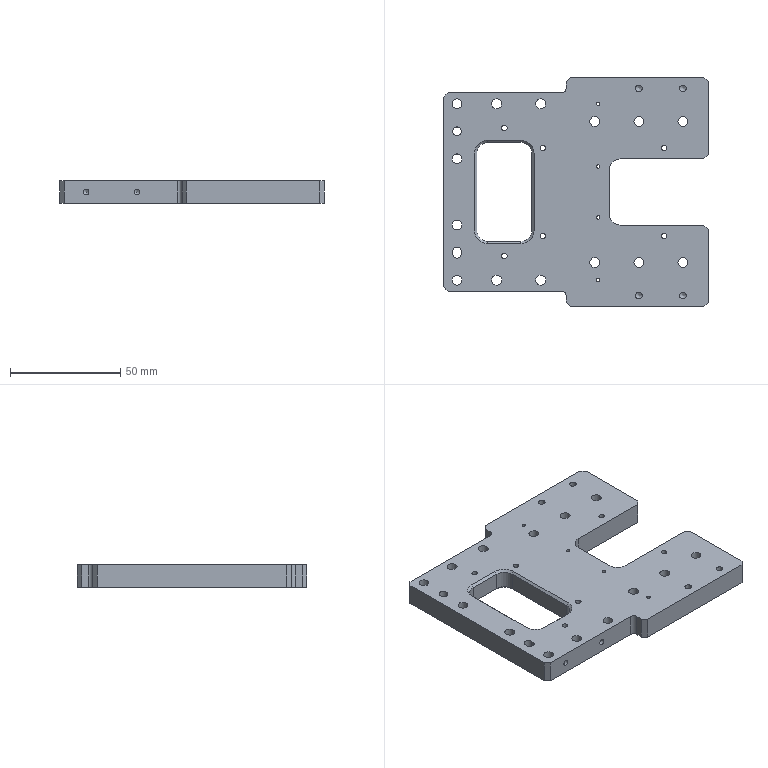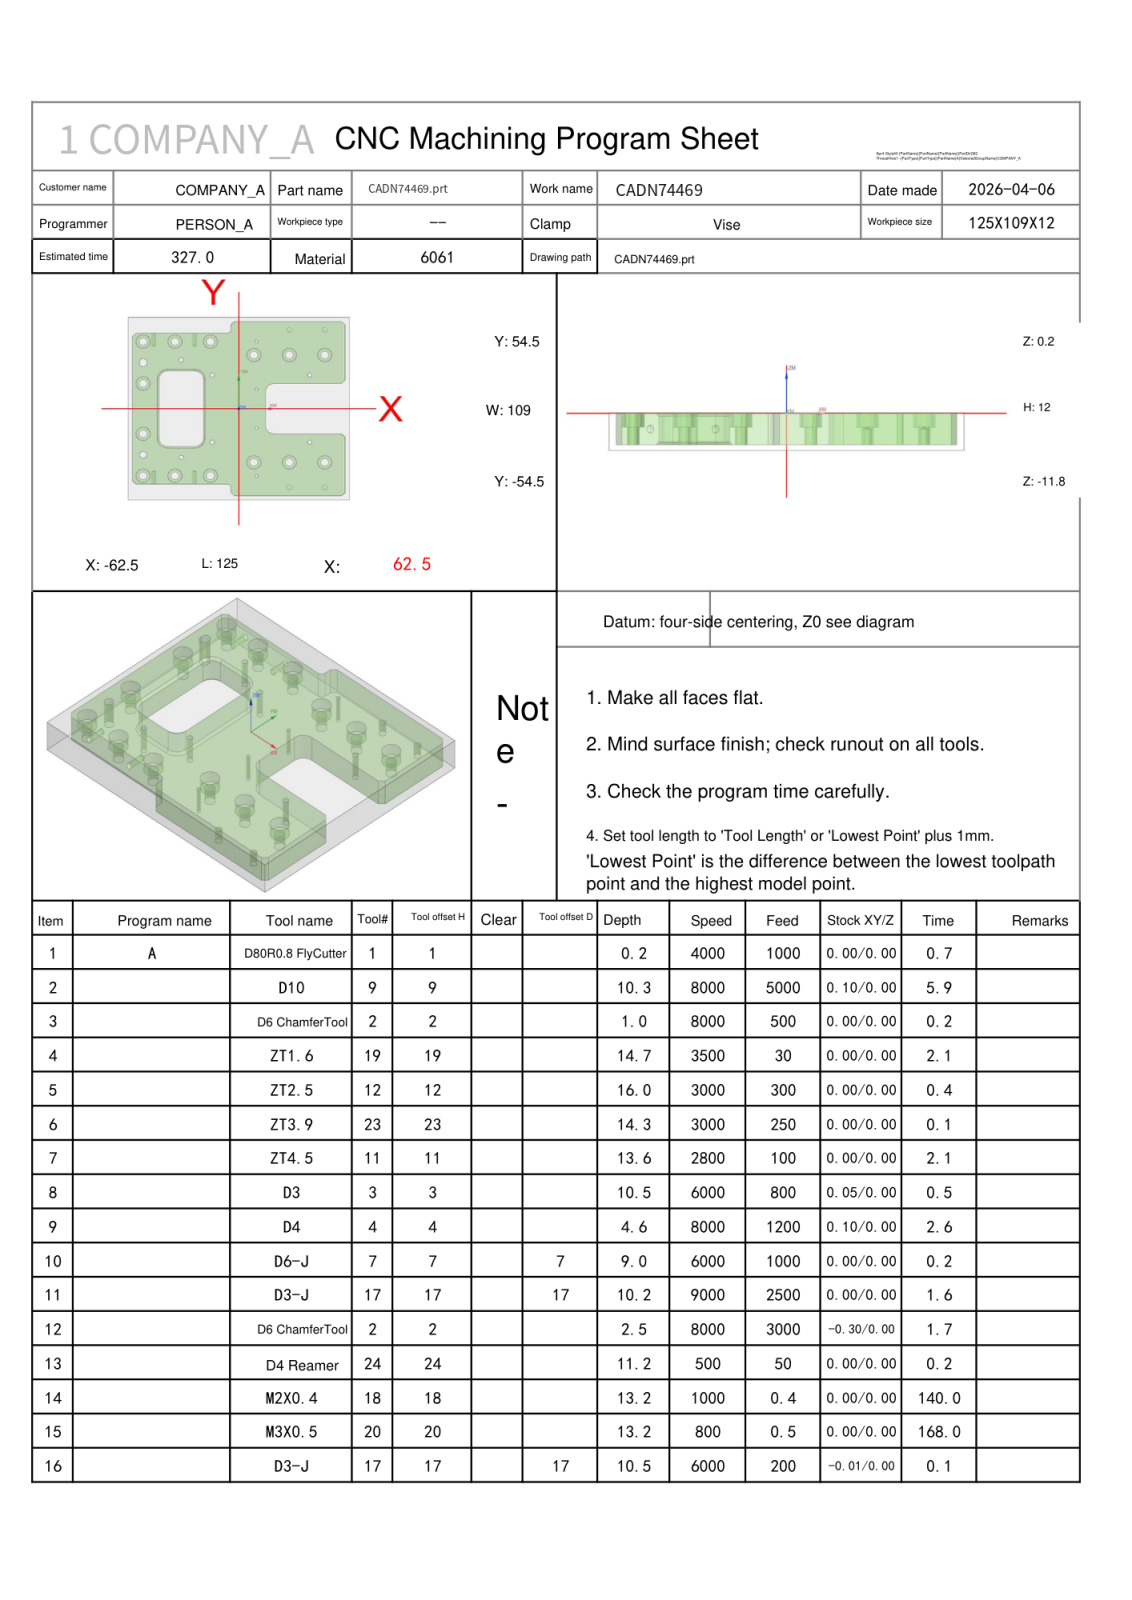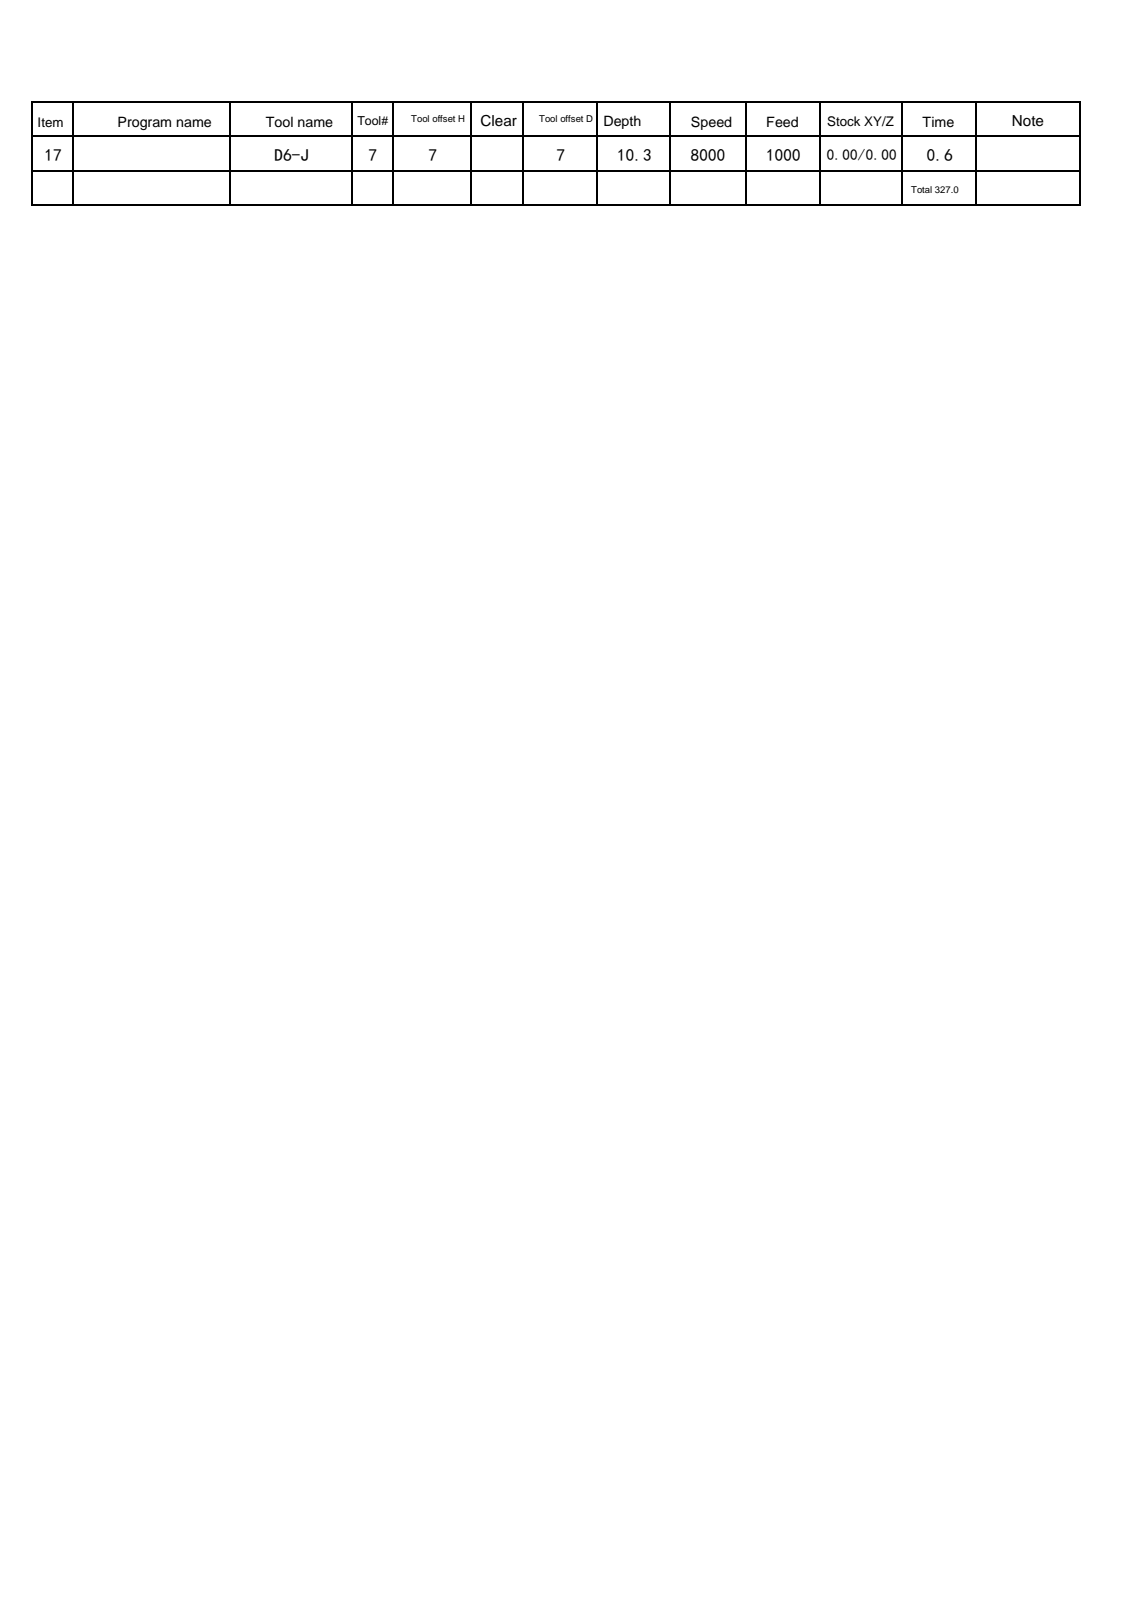NC program | NX | posted by the shop | part box 120 x 104 x 10 mm
Lines 3518 to 5556 of 6435, first 1386 of 2039 lines:
N11 T17 M06
(D3-J  D=3. R=0. H=17 ce=0.00 di=0.00)
G00 G90 G54 X-54. Y15. M03 S8000
G43 H17 Z20.
M08
Z.5
G41 D17
G01 X-53.968 Y14.803 F500.
G03 X-52.742 Y13.758 I1.226 J.197
X-51.5 Y15. I0.0 J1.242
X-51.52 Y14.687 Z-4.4 I-2.5 J0.0
X-51.5 Y15. I-2.48 J.313
X-54. Y17.5 I-2.5 J0.0
X-56.5 Y15. I0.0 J-2.5
X-54. Y12.5 I2.5 J0.0
X-51.52 Y14.687 I0.0 J2.5
G01 X-51.51 Y14.842
G03 X-52.752 Y16.084 I-1.242 J0.0
X-53.944 Y15.192 I0.0 J-1.242
G01 G40 X-54. Y15.
G00 Z20.
Y40.
Z.5
G41 D17
G01 X-53.968 Y39.803
G03 X-52.742 Y38.758 I1.226 J.197
X-51.5 Y40. I0.0 J1.242
X-51.52 Y39.687 Z-4.4 I-2.5 J0.0
X-51.5 Y40. I-2.48 J.313
X-54. Y42.5 I-2.5 J0.0
X-56.5 Y40. I0.0 J-2.5
X-54. Y37.5 I2.5 J0.0
X-51.52 Y39.687 I0.0 J2.5
G01 X-51.51 Y39.842
G03 X-52.752 Y41.084 I-1.242 J0.0
X-53.944 Y40.192 I0.0 J-1.242
G01 G40 X-54. Y40.
G00 Z20.
X-36.
Z.5
G41 D17
G01 X-35.968 Y39.803
G03 X-34.742 Y38.758 I1.226 J.197
X-33.5 Y40. I0.0 J1.242
X-33.52 Y39.687 Z-4.4 I-2.5 J0.0
X-33.5 Y40. I-2.48 J.313
X-36. Y42.5 I-2.5 J0.0
X-38.5 Y40. I0.0 J-2.5
X-36. Y37.5 I2.5 J0.0
X-33.52 Y39.687 I0.0 J2.5
G01 X-33.51 Y39.842
G03 X-34.752 Y41.084 I-1.242 J0.0
X-35.944 Y40.192 I0.0 J-1.242
G01 G40 X-36. Y40.
G00 Z20.
X-16.
Z.5
G41 D17
G01 X-15.968 Y39.803
G03 X-14.742 Y38.758 I1.226 J.197
X-13.5 Y40. I0.0 J1.242
X-13.52 Y39.687 Z-4.4 I-2.5 J0.0
X-13.5 Y40. I-2.48 J.313
X-16. Y42.5 I-2.5 J0.0
X-18.5 Y40. I0.0 J-2.5
X-16. Y37.5 I2.5 J0.0
X-13.52 Y39.687 I0.0 J2.5
G01 X-13.51 Y39.842
G03 X-14.752 Y41.084 I-1.242 J0.0
X-15.944 Y40.192 I0.0 J-1.242
G01 G40 X-16. Y40.
G00 Z20.
X8.5 Y32.
Z.5
G41 D17
G01 X8.532 Y31.803
G03 X9.758 Y30.758 I1.226 J.197
X11. Y32. I0.0 J1.242
X10.98 Y31.687 Z-4.4 I-2.5 J0.0
X11. Y32. I-2.48 J.313
X8.5 Y34.5 I-2.5 J0.0
X6. Y32. I0.0 J-2.5
X8.5 Y29.5 I2.5 J0.0
X10.98 Y31.687 I0.0 J2.5
G01 X10.99 Y31.842
G03 X9.748 Y33.084 I-1.242 J0.0
X8.556 Y32.192 I0.0 J-1.242
G01 G40 X8.5 Y32.
G00 Z20.
X28.5
Z.5
G41 D17
G01 X28.532 Y31.803
G03 X29.758 Y30.758 I1.226 J.197
X31. Y32. I0.0 J1.242
X30.98 Y31.687 Z-4.4 I-2.5 J0.0
X31. Y32. I-2.48 J.313
X28.5 Y34.5 I-2.5 J0.0
X26. Y32. I0.0 J-2.5
X28.5 Y29.5 I2.5 J0.0
X30.98 Y31.687 I0.0 J2.5
G01 X30.99 Y31.842
G03 X29.748 Y33.084 I-1.242 J0.0
X28.556 Y32.192 I0.0 J-1.242
G01 G40 X28.5 Y32.
G00 Z20.
X48.5
Z.5
G41 D17
G01 X48.532 Y31.803
G03 X49.758 Y30.758 I1.226 J.197
X51. Y32. I0.0 J1.242
X50.98 Y31.687 Z-4.4 I-2.5 J0.0
X51. Y32. I-2.48 J.313
X48.5 Y34.5 I-2.5 J0.0
X46. Y32. I0.0 J-2.5
X48.5 Y29.5 I2.5 J0.0
X50.98 Y31.687 I0.0 J2.5
G01 X50.99 Y31.842
G03 X49.748 Y33.084 I-1.242 J0.0
X48.556 Y32.192 I0.0 J-1.242
G01 G40 X48.5 Y32.
G00 Z20.
Y-32.
Z.5
G41 D17
G01 X48.532 Y-32.197
G03 X49.758 Y-33.242 I1.226 J.197
X51. Y-32. I0.0 J1.242
X50.98 Y-32.313 Z-4.4 I-2.5 J0.0
X51. Y-32. I-2.48 J.313
X48.5 Y-29.5 I-2.5 J0.0
X46. Y-32. I0.0 J-2.5
X48.5 Y-34.5 I2.5 J0.0
X50.98 Y-32.313 I0.0 J2.5
G01 X50.99 Y-32.158
G03 X49.748 Y-30.916 I-1.242 J0.0
X48.556 Y-31.808 I0.0 J-1.242
G01 G40 X48.5 Y-32.
G00 Z20.
X28.5
Z.5
G41 D17
G01 X28.532 Y-32.197
G03 X29.758 Y-33.242 I1.226 J.197
X31. Y-32. I0.0 J1.242
X30.98 Y-32.313 Z-4.4 I-2.5 J0.0
X31. Y-32. I-2.48 J.313
X28.5 Y-29.5 I-2.5 J0.0
X26. Y-32. I0.0 J-2.5
X28.5 Y-34.5 I2.5 J0.0
X30.98 Y-32.313 I0.0 J2.5
G01 X30.99 Y-32.158
G03 X29.748 Y-30.916 I-1.242 J0.0
X28.556 Y-31.808 I0.0 J-1.242
G01 G40 X28.5 Y-32.
G00 Z20.
X8.5
Z.5
G41 D17
G01 X8.532 Y-32.197
G03 X9.758 Y-33.242 I1.226 J.197
X11. Y-32. I0.0 J1.242
X10.98 Y-32.313 Z-4.4 I-2.5 J0.0
X11. Y-32. I-2.48 J.313
X8.5 Y-29.5 I-2.5 J0.0
X6. Y-32. I0.0 J-2.5
X8.5 Y-34.5 I2.5 J0.0
X10.98 Y-32.313 I0.0 J2.5
G01 X10.99 Y-32.158
G03 X9.748 Y-30.916 I-1.242 J0.0
X8.556 Y-31.808 I0.0 J-1.242
G01 G40 X8.5 Y-32.
G00 Z20.
X-16. Y-40.
Z.5
G41 D17
G01 X-15.968 Y-40.197
G03 X-14.742 Y-41.242 I1.226 J.197
X-13.5 Y-40. I0.0 J1.242
X-13.52 Y-40.313 Z-4.4 I-2.5 J0.0
X-13.5 Y-40. I-2.48 J.313
X-16. Y-37.5 I-2.5 J0.0
X-18.5 Y-40. I0.0 J-2.5
X-16. Y-42.5 I2.5 J0.0
X-13.52 Y-40.313 I0.0 J2.5
G01 X-13.51 Y-40.158
G03 X-14.752 Y-38.916 I-1.242 J0.0
X-15.944 Y-39.808 I0.0 J-1.242
G01 G40 X-16. Y-40.
G00 Z20.
X-36.
Z.5
G41 D17
G01 X-35.968 Y-40.197
G03 X-34.742 Y-41.242 I1.226 J.197
X-33.5 Y-40. I0.0 J1.242
X-33.52 Y-40.313 Z-4.4 I-2.5 J0.0
X-33.5 Y-40. I-2.48 J.313
X-36. Y-37.5 I-2.5 J0.0
X-38.5 Y-40. I0.0 J-2.5
X-36. Y-42.5 I2.5 J0.0
X-33.52 Y-40.313 I0.0 J2.5
G01 X-33.51 Y-40.158
G03 X-34.752 Y-38.916 I-1.242 J0.0
X-35.944 Y-39.808 I0.0 J-1.242
G01 G40 X-36. Y-40.
G00 Z20.
X-54.
Z.5
G41 D17
G01 X-53.968 Y-40.197
G03 X-52.742 Y-41.242 I1.226 J.197
X-51.5 Y-40. I0.0 J1.242
X-51.52 Y-40.313 Z-4.4 I-2.5 J0.0
X-51.5 Y-40. I-2.48 J.313
X-54. Y-37.5 I-2.5 J0.0
X-56.5 Y-40. I0.0 J-2.5
X-54. Y-42.5 I2.5 J0.0
X-51.52 Y-40.313 I0.0 J2.5
G01 X-51.51 Y-40.158
G03 X-52.752 Y-38.916 I-1.242 J0.0
X-53.944 Y-39.808 I0.0 J-1.242
G01 G40 X-54. Y-40.
G00 Z20.
Y-15.
Z.5
G41 D17
G01 X-53.968 Y-15.197
G03 X-52.742 Y-16.242 I1.226 J.197
X-51.5 Y-15. I0.0 J1.242
X-51.52 Y-15.313 Z-4.4 I-2.5 J0.0
X-51.5 Y-15. I-2.48 J.313
X-54. Y-12.5 I-2.5 J0.0
X-56.5 Y-15. I0.0 J-2.5
X-54. Y-17.5 I2.5 J0.0
X-51.52 Y-15.313 I0.0 J2.5
G01 X-51.51 Y-15.158
G03 X-52.752 Y-13.916 I-1.242 J0.0
X-53.944 Y-14.808 I0.0 J-1.242
G01 G40 X-54. Y-15.
G00 Z20.
G00 G90 X-6.418 Y-50.462 M03 S9000
Z20.
Z.157
G01 X-6.413 Y-50.461 Z.093 F2000.
X-6.399 Y-50.457 Z.035
X-6.377 Y-50.451 Z-.018
X-6.349 Y-50.443 Z-.065
X-6.316 Y-50.432 Z-.107
X-6.279 Y-50.418 Z-.143
X-6.239 Y-50.402 Z-.175
X-6.199 Y-50.383 Z-.203
X-6.159 Y-50.361 Z-.226
X-6.12 Y-50.337 Z-.245
X-6.084 Y-50.309 Z-.261
X-6.052 Y-50.279 Z-.273
X-6.026 Y-50.245 Z-.282
X-6.007 Y-50.208 Z-.288
X-5.996 Y-50.168 Z-.292
X-5.995 Y-50.125 Z-.293
X-6. Y-50. F2500.
Y-47.
G03 X-6.5 Y-46.5 I-.5 J0.0
G01 X-9.625
X-9.654 Y-46.516 Z-.294
X-9.659 Y-46.562 Z-.296
X-9.643 Y-46.634 Z-.3
X-9.607 Y-46.73 Z-.306
X-9.552 Y-46.846 Z-.312
X-9.482 Y-46.979 Z-.32
X-9.3 Y-47.279 Z-.339
X-9.172 Y-47.473 Z-.351
X-8.946 Y-47.789 Z-.372
X-8.572 Y-48.249 Z-.405
X-8.162 Y-48.686 Z-.439
X-7.723 Y-49.094 Z-.473
X-7.264 Y-49.464 Z-.506
X-6.95 Y-49.685 Z-.527
X-6.756 Y-49.812 Z-.539
X-6.459 Y-49.989 Z-.558
X-6.327 Y-50.058 Z-.565
X-6.213 Y-50.11 Z-.572
X-6.12 Y-50.145 Z-.578
X-6.05 Y-50.16 Z-.582
X-6.007 Y-50.154 Z-.584
X-5.995 Y-50.125 Z-.585
X-6. Y-50.
Y-47.
G03 X-6.5 Y-46.5 I-.5 J0.0
G01 X-9.625
X-9.654 Y-46.516 Z-.586
X-9.659 Y-46.562 Z-.589
X-9.643 Y-46.634 Z-.593
X-9.607 Y-46.73 Z-.598
X-9.552 Y-46.846 Z-.605
X-9.482 Y-46.979 Z-.613
X-9.3 Y-47.279 Z-.631
X-9.172 Y-47.473 Z-.644
X-8.946 Y-47.789 Z-.665
X-8.572 Y-48.249 Z-.698
X-8.162 Y-48.686 Z-.732
X-7.723 Y-49.094 Z-.766
X-7.264 Y-49.464 Z-.799
X-6.95 Y-49.685 Z-.819
X-6.756 Y-49.812 Z-.832
X-6.459 Y-49.989 Z-.85
X-6.327 Y-50.058 Z-.858
X-6.213 Y-50.11 Z-.865
X-6.12 Y-50.145 Z-.87
X-6.05 Y-50.16 Z-.874
X-6.007 Y-50.154 Z-.877
X-5.995 Y-50.125 Z-.878
X-6. Y-50.
Y-47.
G03 X-6.5 Y-46.5 I-.5 J0.0
G01 X-9.625
X-9.654 Y-46.516 Z-.879
X-9.659 Y-46.562 Z-.881
X-9.643 Y-46.634 Z-.885
X-9.607 Y-46.73 Z-.891
X-9.552 Y-46.846 Z-.898
X-9.482 Y-46.979 Z-.906
X-9.3 Y-47.279 Z-.924
X-9.172 Y-47.473 Z-.936
X-8.946 Y-47.789 Z-.957
X-8.572 Y-48.249 Z-.99
X-8.162 Y-48.686 Z-1.024
X-7.723 Y-49.094 Z-1.058
X-7.264 Y-49.464 Z-1.091
X-6.95 Y-49.685 Z-1.112
X-6.756 Y-49.812 Z-1.124
X-6.459 Y-49.989 Z-1.143
X-6.327 Y-50.058 Z-1.151
X-6.213 Y-50.11 Z-1.158
X-6.12 Y-50.145 Z-1.163
X-6.05 Y-50.16 Z-1.167
X-6.007 Y-50.154 Z-1.17
X-5.995 Y-50.125 Z-1.171
X-6. Y-50.
Y-47.
G03 X-6.5 Y-46.5 I-.5 J0.0
G01 X-9.625
X-9.654 Y-46.516
X-9.659 Y-46.562 Z-1.174
X-9.643 Y-46.634 Z-1.178
X-9.607 Y-46.73 Z-1.184
X-9.552 Y-46.846 Z-1.19
X-9.482 Y-46.979 Z-1.198
X-9.3 Y-47.279 Z-1.217
X-9.172 Y-47.473 Z-1.229
X-8.946 Y-47.789 Z-1.25
X-8.572 Y-48.249 Z-1.283
X-8.162 Y-48.686 Z-1.317
X-7.723 Y-49.094 Z-1.351
X-7.264 Y-49.464 Z-1.384
X-6.95 Y-49.685 Z-1.405
X-6.756 Y-49.812 Z-1.417
X-6.459 Y-49.989 Z-1.436
X-6.327 Y-50.058 Z-1.443
X-6.213 Y-50.11 Z-1.45
X-6.12 Y-50.145 Z-1.456
X-6.05 Y-50.16 Z-1.46
X-6.007 Y-50.154 Z-1.462
X-5.995 Y-50.125 Z-1.463
X-6. Y-50.
Y-47.
G03 X-6.5 Y-46.5 I-.5 J0.0
G01 X-9.625
X-9.654 Y-46.516 Z-1.464
X-9.659 Y-46.562 Z-1.467
X-9.643 Y-46.634 Z-1.471
X-9.607 Y-46.73 Z-1.476
X-9.552 Y-46.846 Z-1.483
X-9.482 Y-46.979 Z-1.491
X-9.3 Y-47.279 Z-1.509
X-9.172 Y-47.473 Z-1.522
X-8.946 Y-47.789 Z-1.542
X-8.572 Y-48.249 Z-1.575
X-8.162 Y-48.686 Z-1.61
X-7.723 Y-49.094 Z-1.644
X-7.264 Y-49.464 Z-1.677
X-6.95 Y-49.685 Z-1.697
X-6.756 Y-49.812 Z-1.71
X-6.459 Y-49.989 Z-1.728
X-6.327 Y-50.058 Z-1.736
X-6.213 Y-50.11 Z-1.743
X-6.12 Y-50.145 Z-1.748
X-6.05 Y-50.16 Z-1.752
X-6.007 Y-50.154 Z-1.755
X-5.995 Y-50.125 Z-1.756
X-6. Y-50.
Y-47.
G03 X-6.5 Y-46.5 I-.5 J0.0
G01 X-9.625
X-9.654 Y-46.516 Z-1.757
X-9.659 Y-46.562 Z-1.759
X-9.643 Y-46.634 Z-1.763
X-9.607 Y-46.73 Z-1.769
X-9.552 Y-46.846 Z-1.776
X-9.482 Y-46.979 Z-1.784
X-9.3 Y-47.279 Z-1.802
X-9.172 Y-47.473 Z-1.814
X-8.946 Y-47.789 Z-1.835
X-8.572 Y-48.249 Z-1.868
X-8.162 Y-48.686 Z-1.902
X-7.723 Y-49.094 Z-1.936
X-7.264 Y-49.464 Z-1.969
X-6.95 Y-49.685 Z-1.99
X-6.756 Y-49.812 Z-2.002
X-6.459 Y-49.989 Z-2.021
X-6.327 Y-50.058 Z-2.029
X-6.213 Y-50.11 Z-2.035
X-6.12 Y-50.145 Z-2.041
X-6.05 Y-50.16 Z-2.045
X-6.007 Y-50.154 Z-2.048
X-5.995 Y-50.125 Z-2.049
X-6. Y-50.
Y-47.
G03 X-6.5 Y-46.5 I-.5 J0.0
G01 X-9.625
X-9.654 Y-46.516
X-9.659 Y-46.562 Z-2.052
X-9.643 Y-46.634 Z-2.056
X-9.607 Y-46.73 Z-2.062
X-9.552 Y-46.846 Z-2.068
X-9.482 Y-46.979 Z-2.076
X-9.3 Y-47.279 Z-2.095
X-9.172 Y-47.473 Z-2.107
X-8.946 Y-47.789 Z-2.128
X-8.572 Y-48.249 Z-2.161
X-8.162 Y-48.686 Z-2.195
X-7.723 Y-49.094 Z-2.229
X-7.264 Y-49.464 Z-2.262
X-6.95 Y-49.685 Z-2.283
X-6.756 Y-49.812 Z-2.295
X-6.459 Y-49.989 Z-2.313
X-6.327 Y-50.058 Z-2.321
X-6.213 Y-50.11 Z-2.328
X-6.12 Y-50.145 Z-2.334
X-6.05 Y-50.16 Z-2.338
X-6.007 Y-50.154 Z-2.34
X-5.995 Y-50.125 Z-2.341
X-6. Y-50.
Y-47.
G03 X-6.5 Y-46.5 I-.5 J0.0
G01 X-9.625
X-9.654 Y-46.516 Z-2.342
X-9.659 Y-46.562 Z-2.345
X-9.643 Y-46.634 Z-2.349
X-9.607 Y-46.73 Z-2.354
X-9.552 Y-46.846 Z-2.361
X-9.482 Y-46.979 Z-2.369
X-9.3 Y-47.279 Z-2.387
X-9.172 Y-47.473 Z-2.4
X-8.946 Y-47.789 Z-2.42
X-8.572 Y-48.249 Z-2.453
X-8.162 Y-48.686 Z-2.488
X-7.723 Y-49.094 Z-2.522
X-7.264 Y-49.464 Z-2.555
X-6.95 Y-49.685 Z-2.575
X-6.756 Y-49.812 Z-2.588
X-6.459 Y-49.989 Z-2.606
X-6.327 Y-50.058 Z-2.614
X-6.213 Y-50.11 Z-2.621
X-6.12 Y-50.145 Z-2.626
X-6.05 Y-50.16 Z-2.63
X-6.007 Y-50.154 Z-2.633
X-5.995 Y-50.125 Z-2.634
X-6. Y-50.
Y-47.
G03 X-6.5 Y-46.5 I-.5 J0.0
G01 X-9.625
X-9.654 Y-46.516 Z-2.635
X-9.659 Y-46.562 Z-2.637
X-9.643 Y-46.634 Z-2.641
X-9.607 Y-46.73 Z-2.647
X-9.552 Y-46.846 Z-2.654
X-9.482 Y-46.979 Z-2.662
X-9.3 Y-47.279 Z-2.68
X-9.172 Y-47.473 Z-2.692
X-8.946 Y-47.789 Z-2.713
X-8.572 Y-48.249 Z-2.746
X-8.162 Y-48.686 Z-2.78
X-7.723 Y-49.094 Z-2.814
X-7.264 Y-49.464 Z-2.847
X-6.95 Y-49.685 Z-2.868
X-6.756 Y-49.812 Z-2.88
X-6.459 Y-49.989 Z-2.899
X-6.327 Y-50.058 Z-2.907
X-6.213 Y-50.11 Z-2.913
X-6.12 Y-50.145 Z-2.919
X-6.05 Y-50.16 Z-2.923
X-6.007 Y-50.154 Z-2.926
X-5.995 Y-50.125
X-6. Y-50.
Y-47.
G03 X-6.5 Y-46.5 I-.5 J0.0
G01 X-9.625
X-9.654 Y-46.516 Z-2.927
X-9.659 Y-46.562 Z-2.93
X-9.643 Y-46.634 Z-2.934
X-9.607 Y-46.73 Z-2.94
X-9.552 Y-46.846 Z-2.946
X-9.482 Y-46.979 Z-2.954
X-9.3 Y-47.279 Z-2.973
X-9.172 Y-47.473 Z-2.985
X-8.946 Y-47.789 Z-3.006
X-8.572 Y-48.249 Z-3.039
X-8.162 Y-48.686 Z-3.073
X-7.723 Y-49.094 Z-3.107
X-7.264 Y-49.464 Z-3.14
X-6.95 Y-49.685 Z-3.161
X-6.756 Y-49.812 Z-3.173
X-6.459 Y-49.989 Z-3.191
X-6.327 Y-50.058 Z-3.199
X-6.213 Y-50.11 Z-3.206
X-6.12 Y-50.145 Z-3.212
X-6.05 Y-50.16 Z-3.216
X-6.007 Y-50.154 Z-3.218
X-5.995 Y-50.125 Z-3.219
X-6. Y-50.
Y-47.
G03 X-6.5 Y-46.5 I-.5 J0.0
G01 X-9.625
X-9.654 Y-46.516 Z-3.22
X-9.659 Y-46.562 Z-3.223
X-9.643 Y-46.634 Z-3.227
X-9.607 Y-46.73 Z-3.232
X-9.552 Y-46.846 Z-3.239
X-9.482 Y-46.979 Z-3.247
X-9.3 Y-47.279 Z-3.265
X-9.172 Y-47.473 Z-3.278
X-8.946 Y-47.789 Z-3.298
X-8.572 Y-48.249 Z-3.331
X-8.162 Y-48.686 Z-3.365
X-7.723 Y-49.094 Z-3.4
X-7.264 Y-49.464 Z-3.433
X-6.95 Y-49.685 Z-3.453
X-6.756 Y-49.812 Z-3.466
X-6.459 Y-49.989 Z-3.484
X-6.327 Y-50.058 Z-3.492
X-6.213 Y-50.11 Z-3.499
X-6.12 Y-50.145 Z-3.504
X-6.05 Y-50.16 Z-3.508
X-6.007 Y-50.154 Z-3.511
X-5.995 Y-50.125 Z-3.512
X-6. Y-50.
Y-47.
G03 X-6.5 Y-46.5 I-.5 J0.0
G01 X-9.625
X-9.654 Y-46.516 Z-3.513
X-9.659 Y-46.562 Z-3.515
X-9.643 Y-46.634 Z-3.519
X-9.607 Y-46.73 Z-3.525
X-9.552 Y-46.846 Z-3.532
X-9.482 Y-46.979 Z-3.539
X-9.3 Y-47.279 Z-3.558
X-9.172 Y-47.473 Z-3.57
X-8.946 Y-47.789 Z-3.591
X-8.572 Y-48.249 Z-3.624
X-8.162 Y-48.686 Z-3.658
X-7.723 Y-49.094 Z-3.692
X-7.264 Y-49.464 Z-3.725
X-6.95 Y-49.685 Z-3.746
X-6.756 Y-49.812 Z-3.758
X-6.459 Y-49.989 Z-3.777
X-6.327 Y-50.058 Z-3.785
X-6.213 Y-50.11 Z-3.791
X-6.12 Y-50.145 Z-3.797
X-6.05 Y-50.16 Z-3.801
X-6.007 Y-50.154 Z-3.804
X-5.995 Y-50.125
X-6. Y-50.
Y-47.
G03 X-6.5 Y-46.5 I-.5 J0.0
G01 X-9.625
X-9.654 Y-46.516 Z-3.805
X-9.659 Y-46.562 Z-3.808
X-9.643 Y-46.634 Z-3.812
X-9.607 Y-46.73 Z-3.817
X-9.552 Y-46.846 Z-3.824
X-9.482 Y-46.979 Z-3.832
X-9.3 Y-47.279 Z-3.851
X-9.172 Y-47.473 Z-3.863
X-8.946 Y-47.789 Z-3.884
X-8.572 Y-48.249 Z-3.917
X-8.162 Y-48.686 Z-3.951
X-7.723 Y-49.094 Z-3.985
X-7.264 Y-49.464 Z-4.018
X-6.95 Y-49.685 Z-4.039
X-6.756 Y-49.812 Z-4.051
X-6.459 Y-49.989 Z-4.069
X-6.327 Y-50.058 Z-4.077
X-6.213 Y-50.11 Z-4.084
X-6.12 Y-50.145 Z-4.09
X-6.05 Y-50.16 Z-4.094
X-6.007 Y-50.154 Z-4.096
X-5.995 Y-50.125 Z-4.097
X-6. Y-50.
Y-47.
G03 X-6.5 Y-46.5 I-.5 J0.0
G01 X-9.625
X-9.654 Y-46.516 Z-4.098
X-9.659 Y-46.562 Z-4.101
X-9.643 Y-46.634 Z-4.105
X-9.607 Y-46.73 Z-4.11
X-9.552 Y-46.846 Z-4.117
X-9.482 Y-46.979 Z-4.125
X-9.3 Y-47.279 Z-4.143
X-9.172 Y-47.473 Z-4.156
X-8.946 Y-47.789 Z-4.176
X-8.572 Y-48.249 Z-4.209
X-8.162 Y-48.686 Z-4.243
X-7.723 Y-49.094 Z-4.277
X-7.264 Y-49.464 Z-4.31
X-6.95 Y-49.685 Z-4.331
X-6.756 Y-49.812 Z-4.344
X-6.459 Y-49.989 Z-4.362
X-6.327 Y-50.058 Z-4.37
X-6.213 Y-50.11 Z-4.377
X-6.12 Y-50.145 Z-4.382
X-6.05 Y-50.16 Z-4.386
X-6.007 Y-50.154 Z-4.389
X-5.995 Y-50.125 Z-4.39
X-6. Y-50.
Y-47.
G03 X-6.5 Y-46.5 I-.5 J0.0
G01 X-9.625
X-9.654 Y-46.516 Z-4.391
X-9.659 Y-46.562 Z-4.393
X-9.643 Y-46.634 Z-4.397
X-9.607 Y-46.73 Z-4.403
X-9.552 Y-46.846 Z-4.41
X-9.482 Y-46.979 Z-4.417
X-9.3 Y-47.279 Z-4.436
X-9.172 Y-47.473 Z-4.448
X-8.946 Y-47.789 Z-4.469
X-8.572 Y-48.249 Z-4.502
X-8.162 Y-48.686 Z-4.536
X-7.723 Y-49.094 Z-4.57
X-7.264 Y-49.464 Z-4.603
X-6.95 Y-49.685 Z-4.624
X-6.756 Y-49.812 Z-4.636
X-6.459 Y-49.989 Z-4.655
X-6.327 Y-50.058 Z-4.663
X-6.213 Y-50.11 Z-4.669
X-6.12 Y-50.145 Z-4.675
X-6.05 Y-50.16 Z-4.679
X-6.007 Y-50.154 Z-4.681
X-5.995 Y-50.125 Z-4.682
X-6. Y-50.
Y-47.
G03 X-6.5 Y-46.5 I-.5 J0.0
G01 X-9.625
X-9.654 Y-46.516 Z-4.683
X-9.659 Y-46.562 Z-4.686
X-9.643 Y-46.634 Z-4.69
X-9.607 Y-46.73 Z-4.695
X-9.552 Y-46.846 Z-4.702
X-9.482 Y-46.979 Z-4.71
X-9.3 Y-47.279 Z-4.728
X-9.172 Y-47.473 Z-4.741
X-8.946 Y-47.789 Z-4.762
X-8.572 Y-48.249 Z-4.795
X-8.162 Y-48.686 Z-4.829
X-7.723 Y-49.094 Z-4.863
X-7.264 Y-49.464 Z-4.896
X-6.95 Y-49.685 Z-4.917
X-6.756 Y-49.812 Z-4.929
X-6.459 Y-49.989 Z-4.947
X-6.327 Y-50.058 Z-4.955
X-6.213 Y-50.11 Z-4.962
X-6.12 Y-50.145 Z-4.967
X-6.05 Y-50.16 Z-4.972
X-6.007 Y-50.154 Z-4.974
X-5.995 Y-50.125 Z-4.975
X-6. Y-50.
Y-47.
G03 X-6.5 Y-46.5 I-.5 J0.0
G01 X-9.625
X-9.654 Y-46.516 Z-4.976
X-9.659 Y-46.562 Z-4.978
X-9.643 Y-46.634 Z-4.983
X-9.607 Y-46.73 Z-4.988
X-9.552 Y-46.846 Z-4.995
X-9.482 Y-46.979 Z-5.003
X-9.3 Y-47.279 Z-5.021
X-9.172 Y-47.473 Z-5.033
X-8.946 Y-47.789 Z-5.054
X-8.572 Y-48.249 Z-5.087
X-8.162 Y-48.686 Z-5.121
X-7.723 Y-49.094 Z-5.155
X-7.264 Y-49.464 Z-5.188
X-6.95 Y-49.685 Z-5.209
X-6.756 Y-49.812 Z-5.222
X-6.459 Y-49.989 Z-5.24
X-6.327 Y-50.058 Z-5.248
X-6.213 Y-50.11 Z-5.255
X-6.12 Y-50.145 Z-5.26
X-6.05 Y-50.16 Z-5.264
X-6.007 Y-50.154 Z-5.267
X-5.995 Y-50.125 Z-5.268
X-6. Y-50.
Y-47.
G03 X-6.5 Y-46.5 I-.5 J0.0
G01 X-9.625
X-9.654 Y-46.516 Z-5.269
X-9.659 Y-46.562 Z-5.271
X-9.643 Y-46.634 Z-5.275
X-9.607 Y-46.73 Z-5.281
X-9.552 Y-46.846 Z-5.287
X-9.482 Y-46.979 Z-5.295
X-9.3 Y-47.279 Z-5.314
X-9.172 Y-47.473 Z-5.326
X-8.946 Y-47.789 Z-5.347
X-8.572 Y-48.249 Z-5.38
X-8.162 Y-48.686 Z-5.414
X-7.723 Y-49.094 Z-5.448
X-7.264 Y-49.464 Z-5.481
X-6.95 Y-49.685 Z-5.502
X-6.756 Y-49.812 Z-5.514
X-6.459 Y-49.989 Z-5.533
X-6.327 Y-50.058 Z-5.54
X-6.213 Y-50.11 Z-5.547
X-6.12 Y-50.145 Z-5.553
X-6.05 Y-50.16 Z-5.557
X-6.007 Y-50.154 Z-5.559
X-5.995 Y-50.125 Z-5.56
X-6. Y-50.
Y-47.
G03 X-6.5 Y-46.5 I-.5 J0.0
G01 X-9.625
X-9.654 Y-46.516 Z-5.561
X-9.659 Y-46.562 Z-5.564
X-9.643 Y-46.634 Z-5.568
X-9.607 Y-46.73 Z-5.573
X-9.552 Y-46.846 Z-5.58
X-9.482 Y-46.979 Z-5.588
X-9.3 Y-47.279 Z-5.606
X-9.172 Y-47.473 Z-5.619
X-8.946 Y-47.789 Z-5.64
X-8.572 Y-48.249 Z-5.673
X-8.162 Y-48.686 Z-5.707
X-7.723 Y-49.094 Z-5.741
X-7.264 Y-49.464 Z-5.774
X-6.95 Y-49.685 Z-5.794
X-6.756 Y-49.812 Z-5.807
X-6.459 Y-49.989 Z-5.825
X-6.327 Y-50.058 Z-5.833
X-6.213 Y-50.11 Z-5.84
X-6.12 Y-50.145 Z-5.845
X-6.05 Y-50.16 Z-5.849
X-6.007 Y-50.154 Z-5.852
X-5.995 Y-50.125 Z-5.853
X-6. Y-50.
Y-47.
G03 X-6.5 Y-46.5 I-.5 J0.0
G01 X-9.625
X-9.654 Y-46.516 Z-5.854
X-9.659 Y-46.562 Z-5.856
X-9.643 Y-46.634 Z-5.86
X-9.607 Y-46.73 Z-5.866
X-9.552 Y-46.846 Z-5.873
X-9.482 Y-46.979 Z-5.881
X-9.3 Y-47.279 Z-5.899
X-9.172 Y-47.473 Z-5.911
X-8.946 Y-47.789 Z-5.932
X-8.572 Y-48.249 Z-5.965
X-8.162 Y-48.686 Z-5.999
X-7.723 Y-49.094 Z-6.033
X-7.264 Y-49.464 Z-6.066
X-6.95 Y-49.685 Z-6.087
X-6.756 Y-49.812 Z-6.099
X-6.459 Y-49.989 Z-6.118
X-6.327 Y-50.058 Z-6.126
X-6.213 Y-50.11 Z-6.133
X-6.12 Y-50.145 Z-6.138
X-6.05 Y-50.16 Z-6.142
X-6.007 Y-50.154 Z-6.145
X-5.995 Y-50.125 Z-6.146
X-6. Y-50.
Y-47.
G03 X-6.5 Y-46.5 I-.5 J0.0
G01 X-9.625
X-9.654 Y-46.516
X-9.659 Y-46.562 Z-6.149
X-9.643 Y-46.634 Z-6.153
X-9.607 Y-46.73 Z-6.159
X-9.552 Y-46.846 Z-6.165
X-9.482 Y-46.979 Z-6.173
X-9.3 Y-47.279 Z-6.192
X-9.172 Y-47.473 Z-6.204
X-8.946 Y-47.789 Z-6.225
X-8.572 Y-48.249 Z-6.258
X-8.162 Y-48.686 Z-6.292
X-7.723 Y-49.094 Z-6.326
X-7.264 Y-49.464 Z-6.359
X-6.95 Y-49.685 Z-6.38
X-6.756 Y-49.812 Z-6.392
X-6.459 Y-49.989 Z-6.411
X-6.327 Y-50.058 Z-6.418
X-6.213 Y-50.11 Z-6.425
X-6.12 Y-50.145 Z-6.431
X-6.05 Y-50.16 Z-6.435
X-6.007 Y-50.154 Z-6.437
X-5.995 Y-50.125 Z-6.438
X-6. Y-50.
Y-47.
G03 X-6.5 Y-46.5 I-.5 J0.0
G01 X-9.625
X-9.654 Y-46.516 Z-6.439
X-9.659 Y-46.562 Z-6.442
X-9.643 Y-46.634 Z-6.446
X-9.607 Y-46.73 Z-6.451
X-9.552 Y-46.846 Z-6.458
X-9.482 Y-46.979 Z-6.466
X-9.3 Y-47.279 Z-6.484
X-9.172 Y-47.473 Z-6.497
X-8.946 Y-47.789 Z-6.517
X-8.572 Y-48.249 Z-6.55
X-8.162 Y-48.686 Z-6.585
X-7.723 Y-49.094 Z-6.619
X-7.264 Y-49.464 Z-6.652
X-6.95 Y-49.685 Z-6.672
X-6.756 Y-49.812 Z-6.685
X-6.459 Y-49.989 Z-6.703
X-6.327 Y-50.058 Z-6.711
X-6.213 Y-50.11 Z-6.718
X-6.12 Y-50.145 Z-6.723
X-6.05 Y-50.16 Z-6.727
X-6.007 Y-50.154 Z-6.73
X-5.995 Y-50.125 Z-6.731
X-6. Y-50.
Y-47.
G03 X-6.5 Y-46.5 I-.5 J0.0
G01 X-9.625
X-9.654 Y-46.516 Z-6.732
X-9.659 Y-46.562 Z-6.734
X-9.643 Y-46.634 Z-6.738
X-9.607 Y-46.73 Z-6.744
X-9.552 Y-46.846 Z-6.751
X-9.482 Y-46.979 Z-6.759
X-9.3 Y-47.279 Z-6.777
X-9.172 Y-47.473 Z-6.789
X-8.946 Y-47.789 Z-6.81
X-8.572 Y-48.249 Z-6.843
X-8.162 Y-48.686 Z-6.877
X-7.723 Y-49.094 Z-6.911
X-7.264 Y-49.464 Z-6.944
X-6.95 Y-49.685 Z-6.965
X-6.756 Y-49.812 Z-6.977
X-6.459 Y-49.989 Z-6.996
X-6.327 Y-50.058 Z-7.004
X-6.213 Y-50.11 Z-7.01
X-6.12 Y-50.145 Z-7.016
X-6.05 Y-50.16 Z-7.02
X-6.007 Y-50.154 Z-7.023
X-5.995 Y-50.125 Z-7.024
X-6. Y-50.
Y-47.
G03 X-6.5 Y-46.5 I-.5 J0.0
G01 X-9.625
X-9.654 Y-46.516
X-9.659 Y-46.562 Z-7.027
X-9.643 Y-46.634 Z-7.031
X-9.607 Y-46.73 Z-7.037
X-9.552 Y-46.846 Z-7.043
X-9.482 Y-46.979 Z-7.051
X-9.3 Y-47.279 Z-7.07
X-9.172 Y-47.473 Z-7.082
X-8.946 Y-47.789 Z-7.103
X-8.572 Y-48.249 Z-7.136
X-8.162 Y-48.686 Z-7.17
X-7.723 Y-49.094 Z-7.204
X-7.264 Y-49.464 Z-7.237
X-6.95 Y-49.685 Z-7.258
X-6.756 Y-49.812 Z-7.27
X-6.459 Y-49.989 Z-7.288
X-6.327 Y-50.058 Z-7.296
X-6.213 Y-50.11 Z-7.303
X-6.12 Y-50.145 Z-7.309
X-6.05 Y-50.16 Z-7.313
X-6.007 Y-50.154 Z-7.315
X-5.995 Y-50.125 Z-7.316
X-6. Y-50.
Y-47.
G03 X-6.5 Y-46.5 I-.5 J0.0
G01 X-9.625
X-9.654 Y-46.516 Z-7.317
X-9.659 Y-46.562 Z-7.32
X-9.643 Y-46.634 Z-7.324
X-9.607 Y-46.73 Z-7.329
X-9.552 Y-46.846 Z-7.336
X-9.482 Y-46.979 Z-7.344
X-9.3 Y-47.279 Z-7.362
X-9.172 Y-47.473 Z-7.375
X-8.946 Y-47.789 Z-7.395
X-8.572 Y-48.249 Z-7.428
X-8.162 Y-48.686 Z-7.463
X-7.723 Y-49.094 Z-7.497
X-7.264 Y-49.464 Z-7.53
X-6.95 Y-49.685 Z-7.55
X-6.756 Y-49.812 Z-7.563
X-6.459 Y-49.989 Z-7.581
X-6.327 Y-50.058 Z-7.589
X-6.213 Y-50.11 Z-7.596
X-6.12 Y-50.145 Z-7.601
X-6.05 Y-50.16 Z-7.605
X-6.007 Y-50.154 Z-7.608
X-5.995 Y-50.125 Z-7.609
X-6. Y-50.
Y-47.
G03 X-6.5 Y-46.5 I-.5 J0.0
G01 X-9.625
X-9.654 Y-46.516 Z-7.61
X-9.659 Y-46.562 Z-7.612
X-9.643 Y-46.634 Z-7.616
X-9.607 Y-46.73 Z-7.622
X-9.552 Y-46.846 Z-7.629
X-9.482 Y-46.979 Z-7.637
X-9.3 Y-47.279 Z-7.655
X-9.172 Y-47.473 Z-7.667
X-8.946 Y-47.789 Z-7.688
X-8.572 Y-48.249 Z-7.721
X-8.162 Y-48.686 Z-7.755
X-7.723 Y-49.094 Z-7.789
X-7.264 Y-49.464 Z-7.822
X-6.95 Y-49.685 Z-7.843
X-6.756 Y-49.812 Z-7.855
X-6.459 Y-49.989 Z-7.874
X-6.327 Y-50.058 Z-7.882
X-6.213 Y-50.11 Z-7.888
X-6.12 Y-50.145 Z-7.894
X-6.05 Y-50.16 Z-7.898
X-6.007 Y-50.154 Z-7.901
X-5.995 Y-50.125
X-6. Y-50.
Y-47.
G03 X-6.5 Y-46.5 I-.5 J0.0
G01 X-9.625
X-9.654 Y-46.516 Z-7.902
X-9.659 Y-46.562 Z-7.905
X-9.643 Y-46.634 Z-7.909
X-9.607 Y-46.73 Z-7.915
X-9.552 Y-46.846 Z-7.921
X-9.482 Y-46.979 Z-7.929
X-9.3 Y-47.279 Z-7.948
X-9.172 Y-47.473 Z-7.96
X-8.946 Y-47.789 Z-7.981
X-8.572 Y-48.249 Z-8.014
X-8.162 Y-48.686 Z-8.048
X-7.723 Y-49.094 Z-8.082
X-7.264 Y-49.464 Z-8.115
X-6.95 Y-49.685 Z-8.136
X-6.756 Y-49.812 Z-8.148
X-6.459 Y-49.989 Z-8.166
X-6.327 Y-50.058 Z-8.174
X-6.213 Y-50.11 Z-8.181
X-6.12 Y-50.145 Z-8.187
X-6.05 Y-50.16 Z-8.191
X-6.007 Y-50.154 Z-8.193
X-5.995 Y-50.125 Z-8.194
X-6. Y-50.
Y-47.
G03 X-6.5 Y-46.5 I-.5 J0.0
G01 X-9.625
X-9.654 Y-46.516 Z-8.195
X-9.659 Y-46.562 Z-8.198
X-9.643 Y-46.634 Z-8.202
X-9.607 Y-46.73 Z-8.207
X-9.552 Y-46.846 Z-8.214
X-9.482 Y-46.979 Z-8.222
X-9.3 Y-47.279 Z-8.24
X-9.172 Y-47.473 Z-8.253
X-8.946 Y-47.789 Z-8.273
X-8.572 Y-48.249 Z-8.306
X-8.162 Y-48.686 Z-8.34
X-7.723 Y-49.094 Z-8.375
X-7.264 Y-49.464 Z-8.408
X-6.95 Y-49.685 Z-8.428
X-6.756 Y-49.812 Z-8.441
X-6.459 Y-49.989 Z-8.459
X-6.327 Y-50.058 Z-8.467
X-6.213 Y-50.11 Z-8.474
X-6.12 Y-50.145 Z-8.479
X-6.05 Y-50.16 Z-8.483
X-6.007 Y-50.154 Z-8.486
X-5.995 Y-50.125 Z-8.487
X-6. Y-50.
Y-47.
G03 X-6.5 Y-46.5 I-.5 J0.0
G01 X-9.625
X-9.654 Y-46.516 Z-8.488
X-9.659 Y-46.562 Z-8.49
X-9.643 Y-46.634 Z-8.494
X-9.607 Y-46.73 Z-8.5
X-9.552 Y-46.846 Z-8.507
X-9.482 Y-46.979 Z-8.514
X-9.3 Y-47.279 Z-8.533
X-9.172 Y-47.473 Z-8.545
X-8.946 Y-47.789 Z-8.566
X-8.572 Y-48.249 Z-8.599
X-8.162 Y-48.686 Z-8.633
X-7.723 Y-49.094 Z-8.667
X-7.264 Y-49.464 Z-8.7
X-6.95 Y-49.685 Z-8.721
X-6.756 Y-49.812 Z-8.733
X-6.459 Y-49.989 Z-8.752
X-6.327 Y-50.058 Z-8.76
X-6.213 Y-50.11 Z-8.766
X-6.12 Y-50.145 Z-8.772
X-6.05 Y-50.16 Z-8.776
X-6.007 Y-50.154 Z-8.779
X-5.995 Y-50.125
X-6. Y-50.
Y-47.
G03 X-6.5 Y-46.5 I-.5 J0.0
G01 X-9.625
X-9.654 Y-46.516 Z-8.78
X-9.659 Y-46.562 Z-8.783
X-9.643 Y-46.634 Z-8.787
X-9.607 Y-46.73 Z-8.792
X-9.552 Y-46.846 Z-8.799
X-9.482 Y-46.979 Z-8.807
X-9.3 Y-47.279 Z-8.826
X-9.172 Y-47.473 Z-8.838
X-8.946 Y-47.789 Z-8.859
X-8.572 Y-48.249 Z-8.892
X-8.162 Y-48.686 Z-8.926
X-7.723 Y-49.094 Z-8.96
X-7.264 Y-49.464 Z-8.993
X-6.95 Y-49.685 Z-9.014
X-6.756 Y-49.812 Z-9.026
X-6.459 Y-49.989 Z-9.044
X-6.327 Y-50.058 Z-9.052
X-6.213 Y-50.11 Z-9.059
X-6.12 Y-50.145 Z-9.065
X-6.05 Y-50.16 Z-9.069
X-6.007 Y-50.154 Z-9.071
X-5.995 Y-50.125 Z-9.072
X-6. Y-50.
Y-47.
G03 X-6.5 Y-46.5 I-.5 J0.0
G01 X-9.625
X-9.654 Y-46.516 Z-9.073
X-9.659 Y-46.562 Z-9.076
X-9.643 Y-46.634 Z-9.08
X-9.607 Y-46.73 Z-9.085
X-9.552 Y-46.846 Z-9.092
X-9.482 Y-46.979 Z-9.1
X-9.3 Y-47.279 Z-9.118
X-9.172 Y-47.473 Z-9.131
X-8.946 Y-47.789 Z-9.151
X-8.572 Y-48.249 Z-9.184
X-8.162 Y-48.686 Z-9.218
X-7.723 Y-49.094 Z-9.252
X-7.264 Y-49.464 Z-9.285
X-6.95 Y-49.685 Z-9.306
X-6.756 Y-49.812 Z-9.319
X-6.459 Y-49.989 Z-9.337
X-6.327 Y-50.058 Z-9.345
X-6.213 Y-50.11 Z-9.352
X-6.12 Y-50.145 Z-9.357
X-6.05 Y-50.16 Z-9.361
X-6.007 Y-50.154 Z-9.364
X-5.995 Y-50.125 Z-9.365
X-6. Y-50.
Y-47.
G03 X-6.5 Y-46.5 I-.5 J0.0
G01 X-9.625
X-9.654 Y-46.516 Z-9.366
X-9.659 Y-46.562 Z-9.368
X-9.643 Y-46.634 Z-9.372
X-9.607 Y-46.73 Z-9.378
X-9.552 Y-46.846 Z-9.385
X-9.482 Y-46.979 Z-9.392
X-9.3 Y-47.279 Z-9.411
X-9.172 Y-47.473 Z-9.423
X-8.946 Y-47.789 Z-9.444
X-8.572 Y-48.249 Z-9.477
X-8.162 Y-48.686 Z-9.511
X-7.723 Y-49.094 Z-9.545
X-7.264 Y-49.464 Z-9.578
X-6.95 Y-49.685 Z-9.599
X-6.756 Y-49.812 Z-9.611
X-6.459 Y-49.989 Z-9.63
X-6.327 Y-50.058 Z-9.638
X-6.213 Y-50.11 Z-9.644
X-6.12 Y-50.145 Z-9.65
X-6.05 Y-50.16 Z-9.654
X-6.007 Y-50.154 Z-9.656
X-5.995 Y-50.125 Z-9.657
X-6. Y-50.
Y-47.
G03 X-6.5 Y-46.5 I-.5 J0.0
G01 X-9.625
X-9.654 Y-46.516 Z-9.658
X-9.659 Y-46.562 Z-9.661
X-9.643 Y-46.634 Z-9.665
X-9.607 Y-46.73 Z-9.67
X-9.552 Y-46.846 Z-9.677
X-9.482 Y-46.979 Z-9.685
X-9.3 Y-47.279 Z-9.703
X-9.172 Y-47.473 Z-9.716
X-8.946 Y-47.789 Z-9.737
X-8.572 Y-48.249 Z-9.77
X-8.162 Y-48.686 Z-9.804
X-7.723 Y-49.094 Z-9.838
X-7.264 Y-49.464 Z-9.871
X-6.95 Y-49.685 Z-9.892
X-6.756 Y-49.812 Z-9.904
X-6.459 Y-49.989 Z-9.922
X-6.327 Y-50.058 Z-9.93
X-6.213 Y-50.11 Z-9.937
X-6.12 Y-50.145 Z-9.942
X-6.05 Y-50.16 Z-9.947
X-6.007 Y-50.154 Z-9.949
X-5.995 Y-50.125 Z-9.95
X-6. Y-50.
Y-47.
G03 X-6.5 Y-46.5 I-.5 J0.0
G01 X-9.625
X-9.667 Y-46.525 Z-9.949
X-9.705 Y-46.559 Z-9.945
X-9.739 Y-46.599 Z-9.938
X-9.77 Y-46.645 Z-9.927
X-9.797 Y-46.695 Z-9.913
X-9.821 Y-46.747 Z-9.895
X-9.842 Y-46.8 Z-9.873
X-9.86 Y-46.853 Z-9.846
X-9.876 Y-46.903 Z-9.814
X-9.888 Y-46.95 Z-9.777
X-9.898 Y-46.992 Z-9.734
X-9.906 Y-47.027 Z-9.685
X-9.911 Y-47.054 Z-9.63
X-9.914 Y-47.071 Z-9.568
X-9.915 Y-47.078 Z-9.5
G00 Z20.
X-9.897 Y47.078
Z.157
G01 Y47.072 Z.089 F2000.
X-9.894 Y47.055 Z.027
X-9.89 Y47.028 Z-.028
X-9.884 Y46.993 Z-.076
X-9.875 Y46.951 Z-.119
X-9.864 Y46.904 Z-.157
X-9.851 Y46.853 Z-.189
X-9.834 Y46.801 Z-.216
X-9.815 Y46.747 Z-.238
X-9.792 Y46.695 Z-.256
X-9.767 Y46.645 Z-.27
X-9.737 Y46.599 Z-.28
X-9.704 Y46.559 Z-.287
X-9.667 Y46.525 Z-.291
X-9.625 Y46.5 Z-.293
X-6.5 F2500.
G03 X-6. Y47. I0.0 J.5
G01 Y50.
X-5.995 Y50.125
X-6.007 Y50.154 Z-.294
X-6.05 Y50.16 Z-.296
X-6.119 Y50.145 Z-.3
X-6.213 Y50.11 Z-.306
X-6.326 Y50.058 Z-.312
X-6.457 Y49.989 Z-.32
X-6.753 Y49.812 Z-.339
X-6.946 Y49.686 Z-.351
X-7.259 Y49.464 Z-.372
X-7.716 Y49.094 Z-.405
X-8.153 Y48.687 Z-.439
X-8.563 Y48.249 Z-.473
X-8.938 Y47.789 Z-.506
X-9.165 Y47.474 Z-.527
X-9.294 Y47.279 Z-.539
X-9.478 Y46.979 Z-.558
X-9.549 Y46.846 Z-.565
X-9.605 Y46.73 Z-.572
X-9.642 Y46.634 Z-.578
X-9.659 Y46.562 Z-.582
X-9.654 Y46.516 Z-.584
X-9.625 Y46.5 Z-.585
X-6.5
G03 X-6. Y47. I0.0 J.5
G01 Y50.
X-5.995 Y50.125
X-6.007 Y50.154 Z-.586
X-6.05 Y50.16 Z-.589
X-6.119 Y50.145 Z-.593
X-6.213 Y50.11 Z-.598
X-6.326 Y50.058 Z-.605
X-6.457 Y49.989 Z-.613
X-6.753 Y49.812 Z-.631
X-6.946 Y49.686 Z-.644
X-7.259 Y49.464 Z-.665
X-7.716 Y49.094 Z-.698
X-8.153 Y48.687 Z-.732
X-8.563 Y48.249 Z-.766
X-8.938 Y47.789 Z-.799
X-9.165 Y47.474 Z-.82
X-9.294 Y47.279 Z-.832
X-9.478 Y46.979 Z-.85
X-9.549 Y46.846 Z-.858
X-9.605 Y46.73 Z-.865
X-9.642 Y46.634 Z-.87
X-9.659 Y46.562 Z-.874
X-9.654 Y46.516 Z-.877
X-9.625 Y46.5 Z-.878
X-6.5
G03 X-6. Y47. I0.0 J.5
G01 Y50.
X-5.995 Y50.125
X-6.007 Y50.154 Z-.879
X-6.05 Y50.16 Z-.881
X-6.119 Y50.145 Z-.885
X-6.213 Y50.11 Z-.891
X-6.326 Y50.058 Z-.898
X-6.457 Y49.989 Z-.906
X-6.753 Y49.812 Z-.924
X-6.946 Y49.686 Z-.936
X-7.259 Y49.464 Z-.957
X-7.716 Y49.094 Z-.99
X-8.153 Y48.687 Z-1.024
X-8.563 Y48.249 Z-1.058
X-8.938 Y47.789 Z-1.091
X-9.165 Y47.474 Z-1.112
X-9.294 Y47.279 Z-1.125
X-9.478 Y46.979 Z-1.143
X-9.549 Y46.846 Z-1.151
X-9.605 Y46.73 Z-1.158
X-9.642 Y46.634 Z-1.163
X-9.659 Y46.562 Z-1.167
X-9.654 Y46.516 Z-1.17
X-9.625 Y46.5 Z-1.171
X-6.5
G03 X-6. Y47. I0.0 J.5
G01 Y50.
X-5.995 Y50.125
X-6.007 Y50.154
X-6.05 Y50.16 Z-1.174
X-6.119 Y50.145 Z-1.178
X-6.213 Y50.11 Z-1.184
X-6.326 Y50.058 Z-1.19
X-6.457 Y49.989 Z-1.198
X-6.753 Y49.812 Z-1.217
X-6.946 Y49.686 Z-1.229
X-7.259 Y49.464 Z-1.25
X-7.716 Y49.094 Z-1.283
X-8.153 Y48.687 Z-1.317
X-8.563 Y48.249 Z-1.351
X-8.938 Y47.789 Z-1.384
X-9.165 Y47.474 Z-1.405
X-9.294 Y47.279 Z-1.417
X-9.478 Y46.979 Z-1.436
X-9.549 Y46.846 Z-1.443
X-9.605 Y46.73 Z-1.45
X-9.642 Y46.634 Z-1.456
X-9.659 Y46.562 Z-1.46
X-9.654 Y46.516 Z-1.462
X-9.625 Y46.5 Z-1.463
X-6.5
G03 X-6. Y47. I0.0 J.5
G01 Y50.
X-5.995 Y50.125
X-6.007 Y50.154 Z-1.464
X-6.05 Y50.16 Z-1.467
X-6.119 Y50.145 Z-1.471
X-6.213 Y50.11 Z-1.476
X-6.326 Y50.058 Z-1.483
X-6.457 Y49.989 Z-1.491
X-6.753 Y49.812 Z-1.509
X-6.946 Y49.686 Z-1.522
X-7.259 Y49.464 Z-1.542
X-7.716 Y49.094 Z-1.575
X-8.153 Y48.687 Z-1.61
X-8.563 Y48.249 Z-1.644
X-8.938 Y47.789 Z-1.677
X-9.165 Y47.474 Z-1.697
X-9.294 Y47.279 Z-1.71
X-9.478 Y46.979 Z-1.728
X-9.549 Y46.846 Z-1.736
X-9.605 Y46.73 Z-1.743
X-9.642 Y46.634 Z-1.748
X-9.659 Y46.562 Z-1.752
X-9.654 Y46.516 Z-1.755
X-9.625 Y46.5 Z-1.756
X-6.5
G03 X-6. Y47. I0.0 J.5
G01 Y50.
X-5.995 Y50.125
X-6.007 Y50.154 Z-1.757
X-6.05 Y50.16 Z-1.759
X-6.119 Y50.145 Z-1.763
X-6.213 Y50.11 Z-1.769
X-6.326 Y50.058 Z-1.776
X-6.457 Y49.989 Z-1.784
X-6.753 Y49.812 Z-1.802
X-6.946 Y49.686 Z-1.814
X-7.259 Y49.464 Z-1.835
X-7.716 Y49.094 Z-1.868
X-8.153 Y48.687 Z-1.902
X-8.563 Y48.249 Z-1.936
X-8.938 Y47.789 Z-1.969
X-9.165 Y47.474 Z-1.99
X-9.294 Y47.279 Z-2.002
X-9.478 Y46.979 Z-2.021
X-9.549 Y46.846 Z-2.029
X-9.605 Y46.73 Z-2.035
X-9.642 Y46.634 Z-2.041
X-9.659 Y46.562 Z-2.045
X-9.654 Y46.516 Z-2.048
X-9.625 Y46.5 Z-2.049
X-6.5
G03 X-6. Y47. I0.0 J.5
G01 Y50.
X-5.995 Y50.125
X-6.007 Y50.154
X-6.05 Y50.16 Z-2.052
X-6.119 Y50.145 Z-2.056
X-6.213 Y50.11 Z-2.062
X-6.326 Y50.058 Z-2.068
X-6.457 Y49.989 Z-2.076
X-6.753 Y49.812 Z-2.095
X-6.946 Y49.686 Z-2.107
X-7.259 Y49.464 Z-2.128
X-7.716 Y49.094 Z-2.161
X-8.153 Y48.687 Z-2.195
X-8.563 Y48.249 Z-2.229
X-8.938 Y47.789 Z-2.262
X-9.165 Y47.474 Z-2.283
X-9.294 Y47.279 Z-2.295
X-9.478 Y46.979 Z-2.313
X-9.549 Y46.846 Z-2.321
X-9.605 Y46.73 Z-2.328
X-9.642 Y46.634 Z-2.334
X-9.659 Y46.562 Z-2.338
X-9.654 Y46.516 Z-2.34
X-9.625 Y46.5 Z-2.341
X-6.5
G03 X-6. Y47. I0.0 J.5
G01 Y50.
X-5.995 Y50.125
X-6.007 Y50.154 Z-2.342
X-6.05 Y50.16 Z-2.345
X-6.119 Y50.145 Z-2.349
X-6.213 Y50.11 Z-2.354
X-6.326 Y50.058 Z-2.361
X-6.457 Y49.989 Z-2.369
X-6.753 Y49.812 Z-2.387
X-6.946 Y49.686 Z-2.4
X-7.259 Y49.464 Z-2.42
X-7.716 Y49.094 Z-2.453
X-8.153 Y48.687 Z-2.488
X-8.563 Y48.249 Z-2.522
X-8.938 Y47.789 Z-2.555
X-9.165 Y47.474 Z-2.575
X-9.294 Y47.279 Z-2.588
X-9.478 Y46.979 Z-2.606
X-9.549 Y46.846 Z-2.614
X-9.605 Y46.73 Z-2.621
X-9.642 Y46.634 Z-2.626
X-9.659 Y46.562 Z-2.63
X-9.654 Y46.516 Z-2.633
X-9.625 Y46.5 Z-2.634
X-6.5
G03 X-6. Y47. I0.0 J.5
G01 Y50.
X-5.995 Y50.125
X-6.007 Y50.154 Z-2.635
X-6.05 Y50.16 Z-2.637
X-6.119 Y50.145 Z-2.641
X-6.213 Y50.11 Z-2.647
X-6.326 Y50.058 Z-2.654
X-6.457 Y49.989 Z-2.662
X-6.753 Y49.812 Z-2.68
X-6.946 Y49.686 Z-2.692
X-7.259 Y49.464 Z-2.713
X-7.716 Y49.094 Z-2.746
X-8.153 Y48.687 Z-2.78
X-8.563 Y48.249 Z-2.814
X-8.938 Y47.789 Z-2.847
X-9.165 Y47.474 Z-2.868
X-9.294 Y47.279 Z-2.88
X-9.478 Y46.979 Z-2.899
X-9.549 Y46.846 Z-2.907
X-9.605 Y46.73 Z-2.913